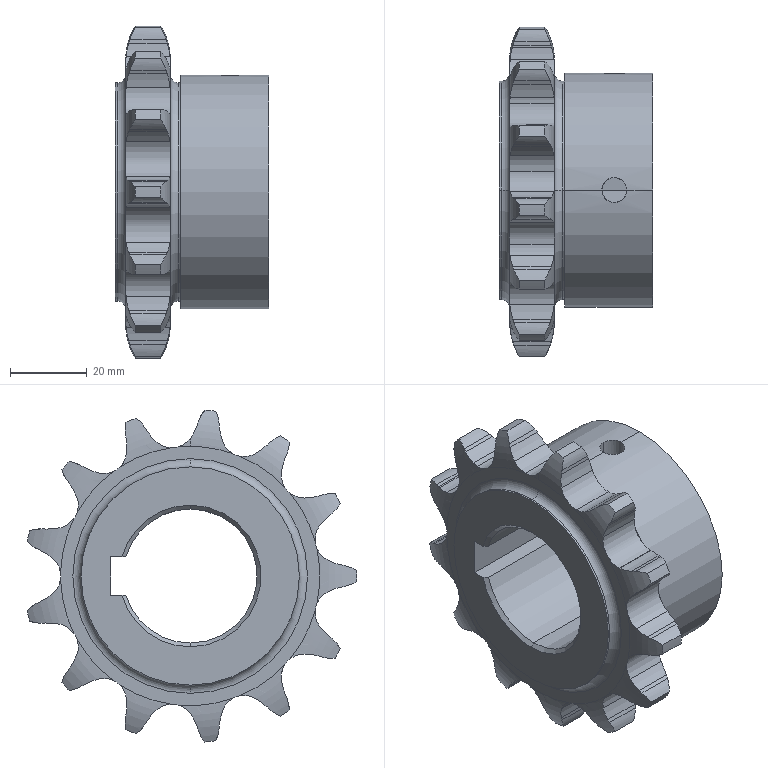Part | SolidWorks | features BaseBody 1 | 1 solid | 170 faces | box 40 x 86.057 x 86.665 mm | volume 91604 mm3 | cylinder 98 | plane 34 | torus 32 | cone 6 | commonest cylinder face diameters 17.67 x28 31.126 x27 12.07 x17 87 x13 6.5 x4 57 x4